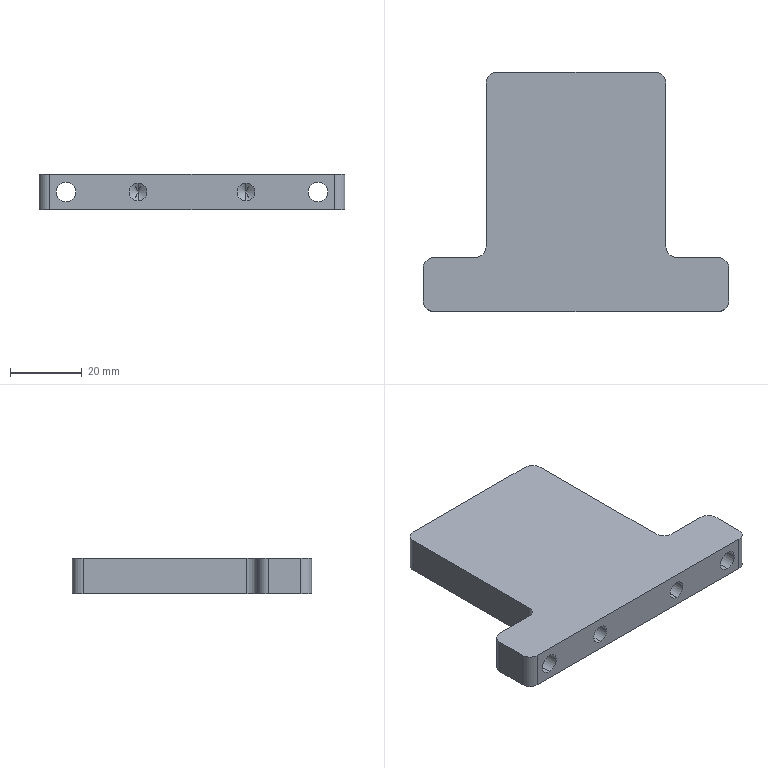Part | STEP file | 1 solid | 50 faces | box 85 x 66.5 x 10 mm | volume 36549 mm3 | cylinder 26 | cone 14 | plane 10 | commonest cylinder face diameters 5 x8 6 x8 4.2 x6 5.5 x4